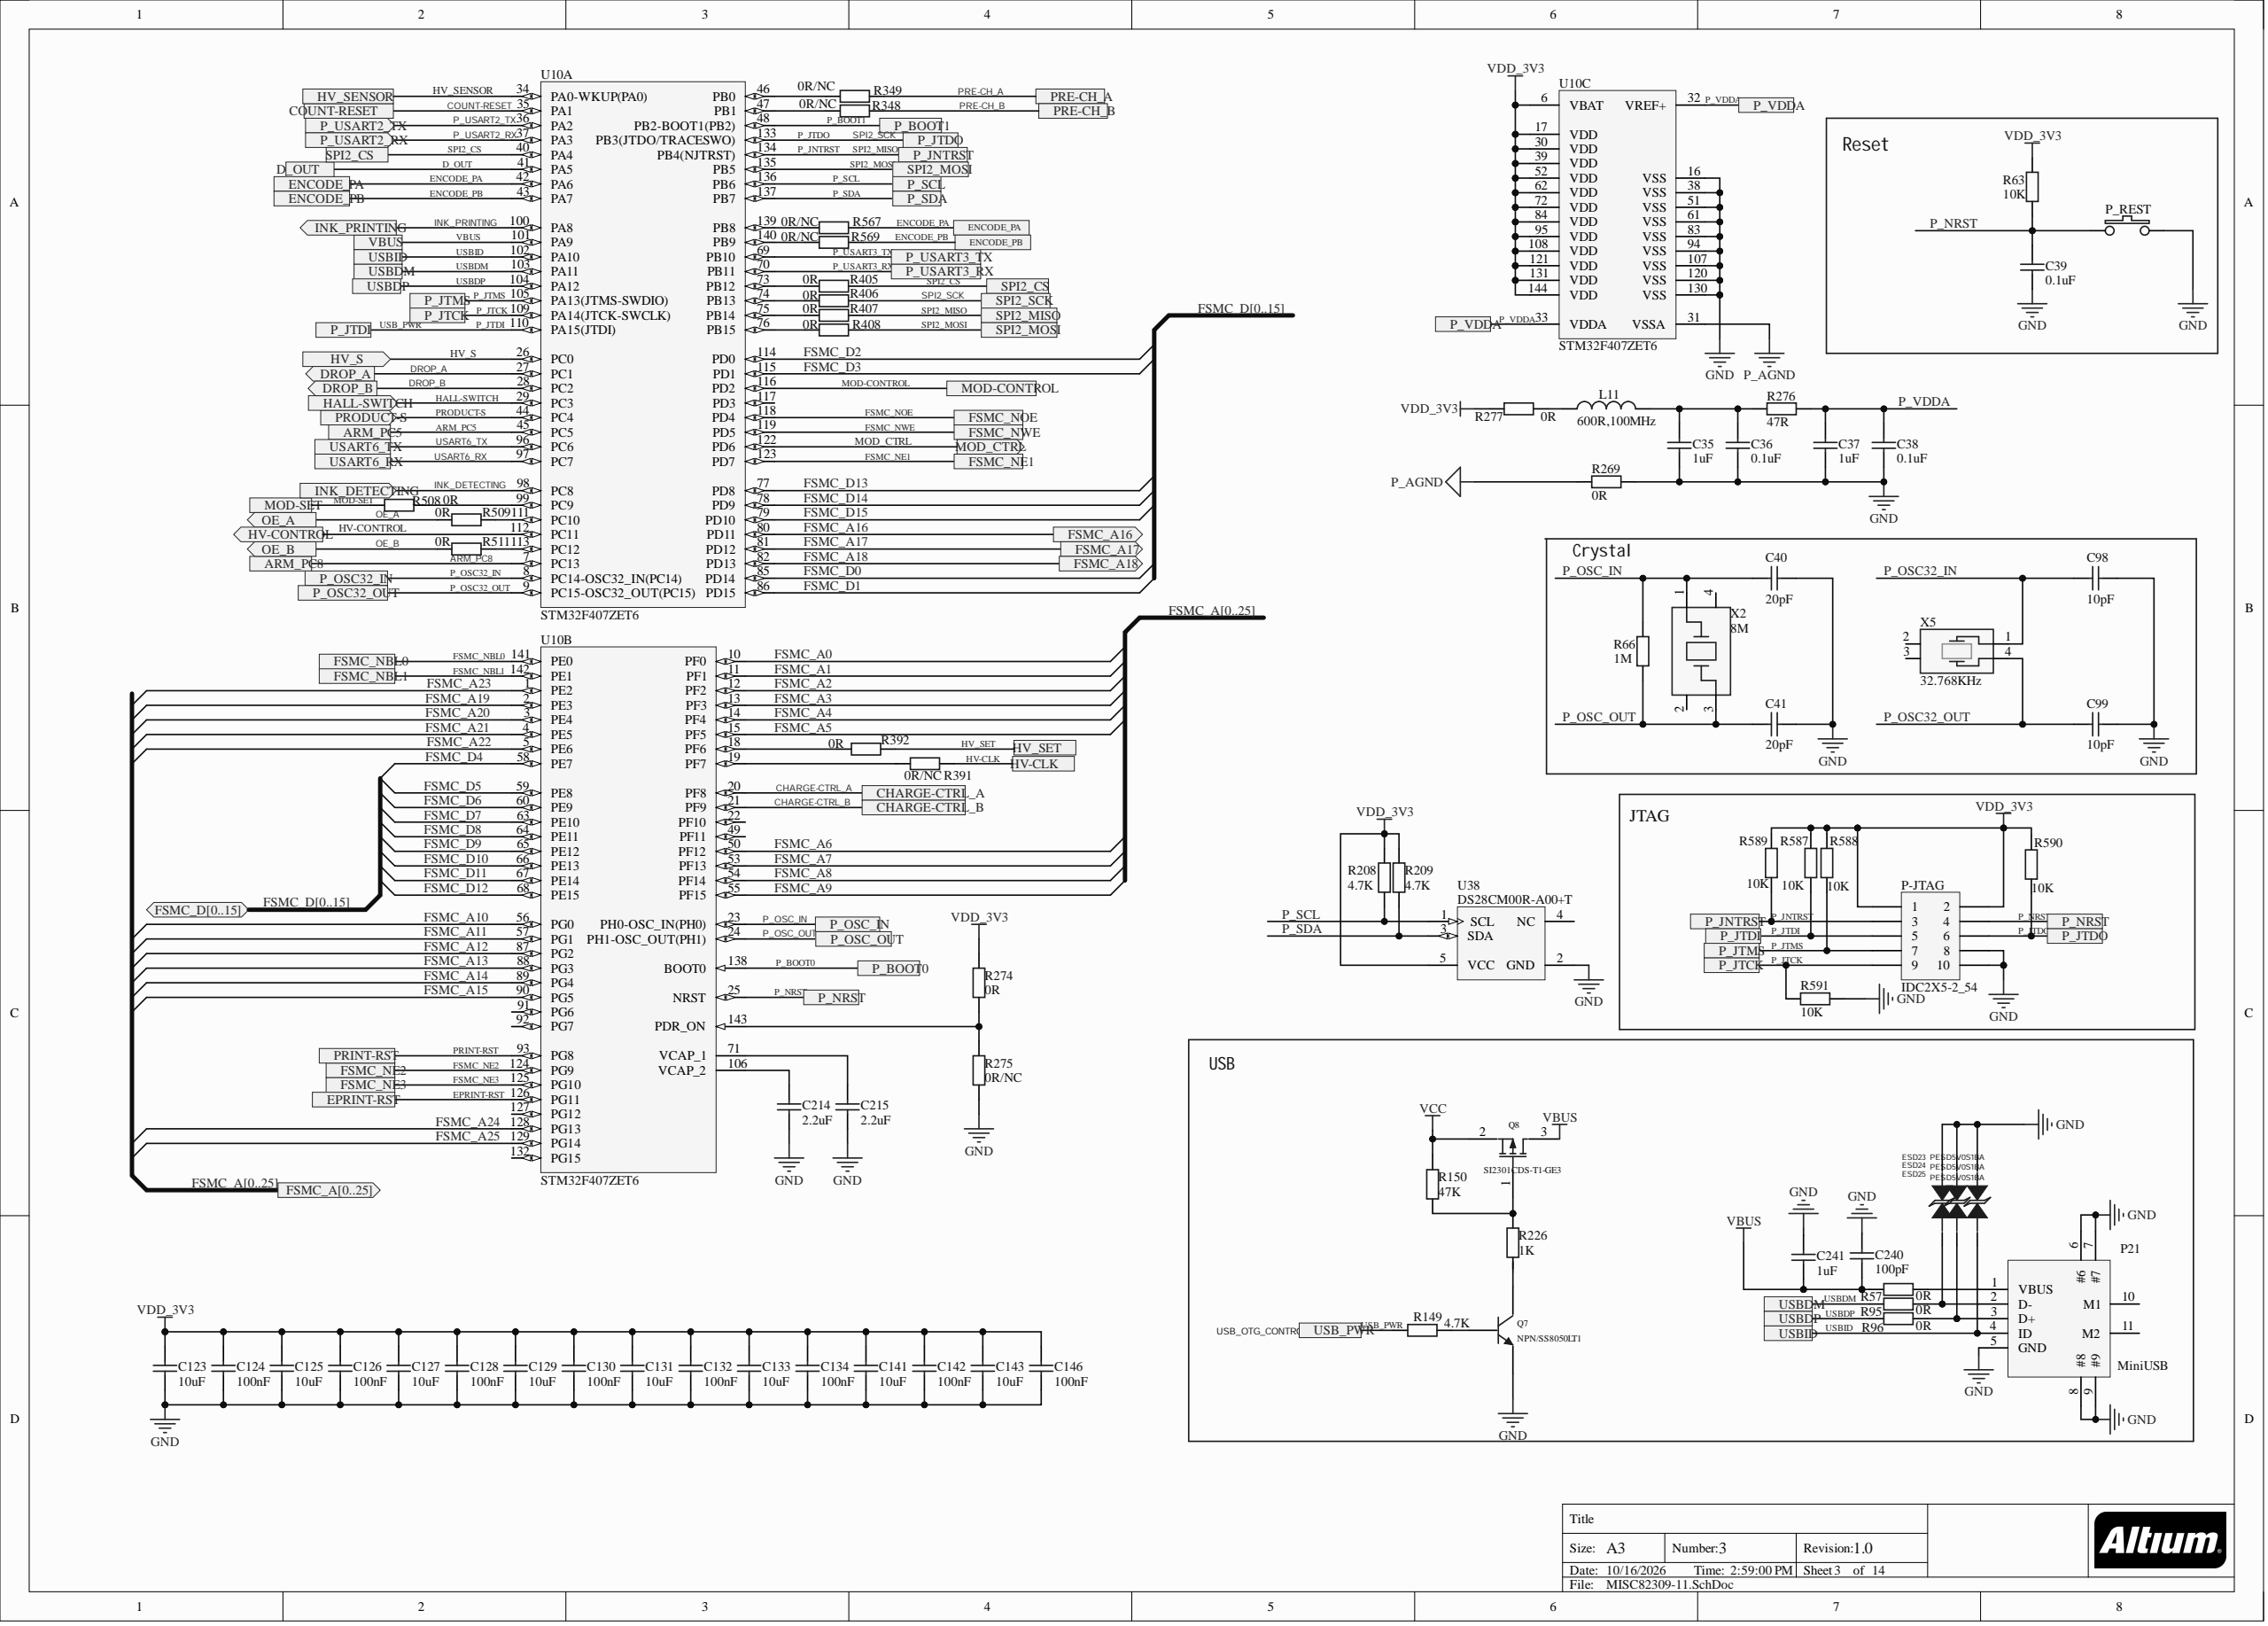Circuit board | Altium Designer | 747 parts | 576 nets | one sheet of the schematic
Parts on this sheet (reference | value | footprint):
C35 | 1uF | CAP_0805
C36 | 0.1uF | CAP_0805
C37 | 1uF | CAP_0805
C38 | 0.1uF | CAP_0805
C39 | 0.1uF | C0603
C40 | 20pF | C0603
C41 | 20pF | C0603
C98 | 10pF | C0603
C99 | 10pF | C0603
C123 | 10uF | C0805
C124 | 100nF | C0805
C125 | 10uF | C0805
C126 | 100nF | C0805
C127 | 10uF | C0805
C128 | 100nF | C0805
C129 | 10uF | C0805
C130 | 100nF | C0805
C131 | 10uF | C0805
C132 | 100nF | C0805
C133 | 10uF | C0805
C134 | 100nF | C0805
C141 | 10uF | C0805
C142 | 100nF | C0805
C143 | 10uF | C0805
C146 | 100nF | C0805
C214 | 2.2uF | CAP_0805
C215 | 2.2uF | CAP_0805
C240 | 100pF | C0603
C241 | 1uF | C0603
ESD23 | PESD5V0S1BA | SOD323
ESD24 | PESD5V0S1BA | SOD323
ESD25 | PESD5V0S1BA | SOD323
L11 | 600R,100MHz | R0805
P21 | MiniUSB | MiniUSB-A
P-JTAG | IDC2X5-2_54 | IDC2X5-2_54
P_REST | SW | SW-6X3X2.5
Q7 | NPN/SS8050LT1 | SOT-23-3
Q8 | SI2301CDS-T1-GE3 | SOT-23
R57 | 0R | RES_0603
R63 | 10K | R0603
R66 | 1M | R0603
R95 | 0R | RES_0603
R96 | 0R | RES_0603
R149 | 4.7K | R0603
R150 | 47K | RES_0603
R208 | 4.7K | R0603
R209 | 4.7K | R0603
R226 | 1K | RES_0603
R269 | 0R | R0805
R274 | 0R | RES_0603
R275 | 0R/NC | RES_0603
R276 | 47R | R0805
R277 | 0R | R0805
R348 | 0R/NC | RES_0603
R349 | 0R/NC | RES_0603
R392 | 0R | RES_0603
R405 | 0R | RES_0603
R406 | 0R | RES_0603
R407 | 0R | RES_0603
R408 | 0R | RES_0603
R508 | 0R | RES_0603
R509 | 0R | RES_0603
R511 | 0R | RES_0603
R567 | 0R/NC | RES_0603
R569 | 0R/NC | RES_0603
R587 | 10K | R0603
R588 | 10K | R0603
R589 | 10K | R0603
R590 | 10K | R0603
R591 | 10K | R0603
U10 | STM32F407ZET6 | LQFP144
U38 | DS28CM00R-A00+T | U5+1_N
X2 | 8M | SMD5032
X5 | 32.768KHz | Y_XTAL_T7
Nets of these parts (net: part-pin ...):
VDD_3V3: C123-2 C124-2 C125-2 C126-2 C127-2 C128-2 C129-2 C130-2 C131-2 C132-2 C133-2 C134-2 C141-2 C142-2 C143-2 C146-2 P-JTAG-1 P-JTAG-2 R63-1 R208-1 R209-1 R274-2 R277-1 R587-2 R588-2 R589-2 R590-2 U38-5 U10-6 U10-17 U10-30 U10-39 U10-52 U10-62 U10-72 U10-84 U10-95 U10-108 U10-121 U10-131 U10-144
VCC: Q8-2 R150-2
VBUS: C240-2 C241-2 Q8-3 R57-2 U10-101
USBID: ESD23-1 P21-4 U10-102
USBDP: R96-2 U10-104
USBDM: R95-2 U10-103
USART6_TX: U10-96
USART6_RX: U10-97
SPI2_MOSI: R408-2 U10-135
SPI2_CS: R405-2 U10-40
PRODUCT-S: U10-44
PRINT-RST: U10-93
PRE-CH_B: R348-2
PRE-CH_A: R349-2
P_VDDA: C37-2 C38-2 R276-2 U10-32 U10-33
P_USART3_TX: U10-69
P_USART3_RX: U10-70
P_USART2_TX: U10-36
P_USART2_RX: U10-37
P_SDA: R209-2 U38-3 U10-137
P_SCL: R208-2 U38-1 U10-136
P_OSC_OUT: C41-2 R66-2 X2-3 U10-24
P_OSC_IN: C40-2 R66-1 X2-1 U10-23
P_OSC32_OUT: C99-2 X5-4 U10-9
P_OSC32_IN: C98-2 X5-1 U10-8
P_NRST: C39-2 P-JTAG-4 P_REST-1 R63-2 U10-25
P_JTMS: P-JTAG-7 R588-1 U10-105
P_JTDO: P-JTAG-6 R406-2 R590-1 U10-133
P_JTDI: P-JTAG-5 R149-1 R587-1 U10-110
P_JTCK: P-JTAG-9 R591-2 U10-109
P_JNTRST: P-JTAG-3 R407-2 R589-1 U10-134
P_BOOT1: U10-48
P_BOOT0: U10-138
P_AGND: R269-1 U10-31
OE_B: R511-1
OE_A: R509-1
NetR569_1: R569-1 U10-140
NetR567_1: R567-1 U10-139
NetR511_2: R511-2 U10-113
NetR509_2: R509-2 U10-111
NetR508_1: R508-1 U10-99
NetR408_1: R408-1 U10-76
NetR407_1: R407-1 U10-75
NetR406_1: R406-1 U10-74
NetR405_1: R405-1 U10-73
NetR392_1: R392-1 U10-18
NetR349_1: R349-1 U10-46
NetR348_1: R348-1 U10-47
NetR274_1: R274-1 R275-2 U10-143
NetQ8_1: Q8-1 R150-1 R226-1
NetQ7_3: Q7-3 R226-2
NetQ7_1: Q7-1 R149-2
NetP21_1: P21-1 R57-1
NetL11_1: L11-1 R277-2
NetESD25_1: ESD25-1 P21-3 R96-1
NetESD24_1: ESD24-1 P21-2 R95-1
NetC215_1: C215-1 U10-71
NetC214_1: C214-1 U10-106
NetC35_2: C35-2 C36-2 L11-2 R276-1
MOD_CTRL: U10-122
MOD-SET: R508-2
MOD-CONTROL: U10-116
INK_PRINTING: U10-100
INK_DETECTING: U10-98
HV_SET: R392-2
HV_SENSOR: U10-34
HV_S: U10-26
HV-CONTROL: U10-112
HALL-SWITCH: U10-29
GND: C35-1 C36-1 C37-1 C38-1 C39-1 C40-1 C41-1 C98-1 C99-1 C123-1 C124-1 C125-1 C126-1 C127-1 C128-1 C129-1 C130-1 C131-1 C132-1 C133-1 C134-1 C141-1 C142-1 C143-1 C146-1 C214-2 C215-2 C240-1 C241-1 ESD23-2 ESD24-2 ESD25-2 P21-5 P21-6 P21-7 P21-8 P21-9 P-JTAG-8 P-JTAG-10 P_REST-2 Q7-2 R269-2 R275-1 R591-1 U38-2 U10-16 U10-38 U10-51 U10-61 U10-83 U10-94 U10-107 U10-120 U10-130
FSMC_NWE: U10-119
FSMC_NOE: U10-118
FSMC_NE3: U10-125
FSMC_NE2: U10-124
FSMC_NE1: U10-123
FSMC_NBL1: U10-142
FSMC_NBL0: U10-141
FSMC_D15: U10-79
FSMC_D14: U10-78
FSMC_D13: U10-77
FSMC_D12: U10-68
FSMC_D11: U10-67
FSMC_D10: U10-66
FSMC_D9: U10-65
FSMC_D8: U10-64
FSMC_D7: U10-63
FSMC_D6: U10-60
FSMC_D5: U10-59
FSMC_D4: U10-58
FSMC_D3: U10-115
FSMC_D2: U10-114
FSMC_D1: U10-86
FSMC_D0: U10-85
FSMC_A18: U10-82
FSMC_A17: U10-81
FSMC_A16: U10-80
FSMC_A15: U10-90
FSMC_A14: U10-89
FSMC_A13: U10-88
FSMC_A12: U10-87
FSMC_A11: U10-57
FSMC_A10: U10-56
FSMC_A9: U10-55
FSMC_A8: U10-54
FSMC_A7: U10-53
FSMC_A6: U10-50
FSMC_A5: U10-15
FSMC_A4: U10-14
FSMC_A3: U10-13
FSMC_A2: U10-12
FSMC_A1: U10-11
FSMC_A0: U10-10
EPRINT-RST: U10-126
ENCODE_PB: R569-2 U10-43
ENCODE_PA: R567-2 U10-42
DROP_B: U10-28
DROP_A: U10-27
D_OUT: U10-41
COUNT-RESET: U10-35
CHARGE-CTRL_B: U10-21
CHARGE-CTRL_A: U10-20
ARM_PC8: U10-7
ARM_PC5: U10-45